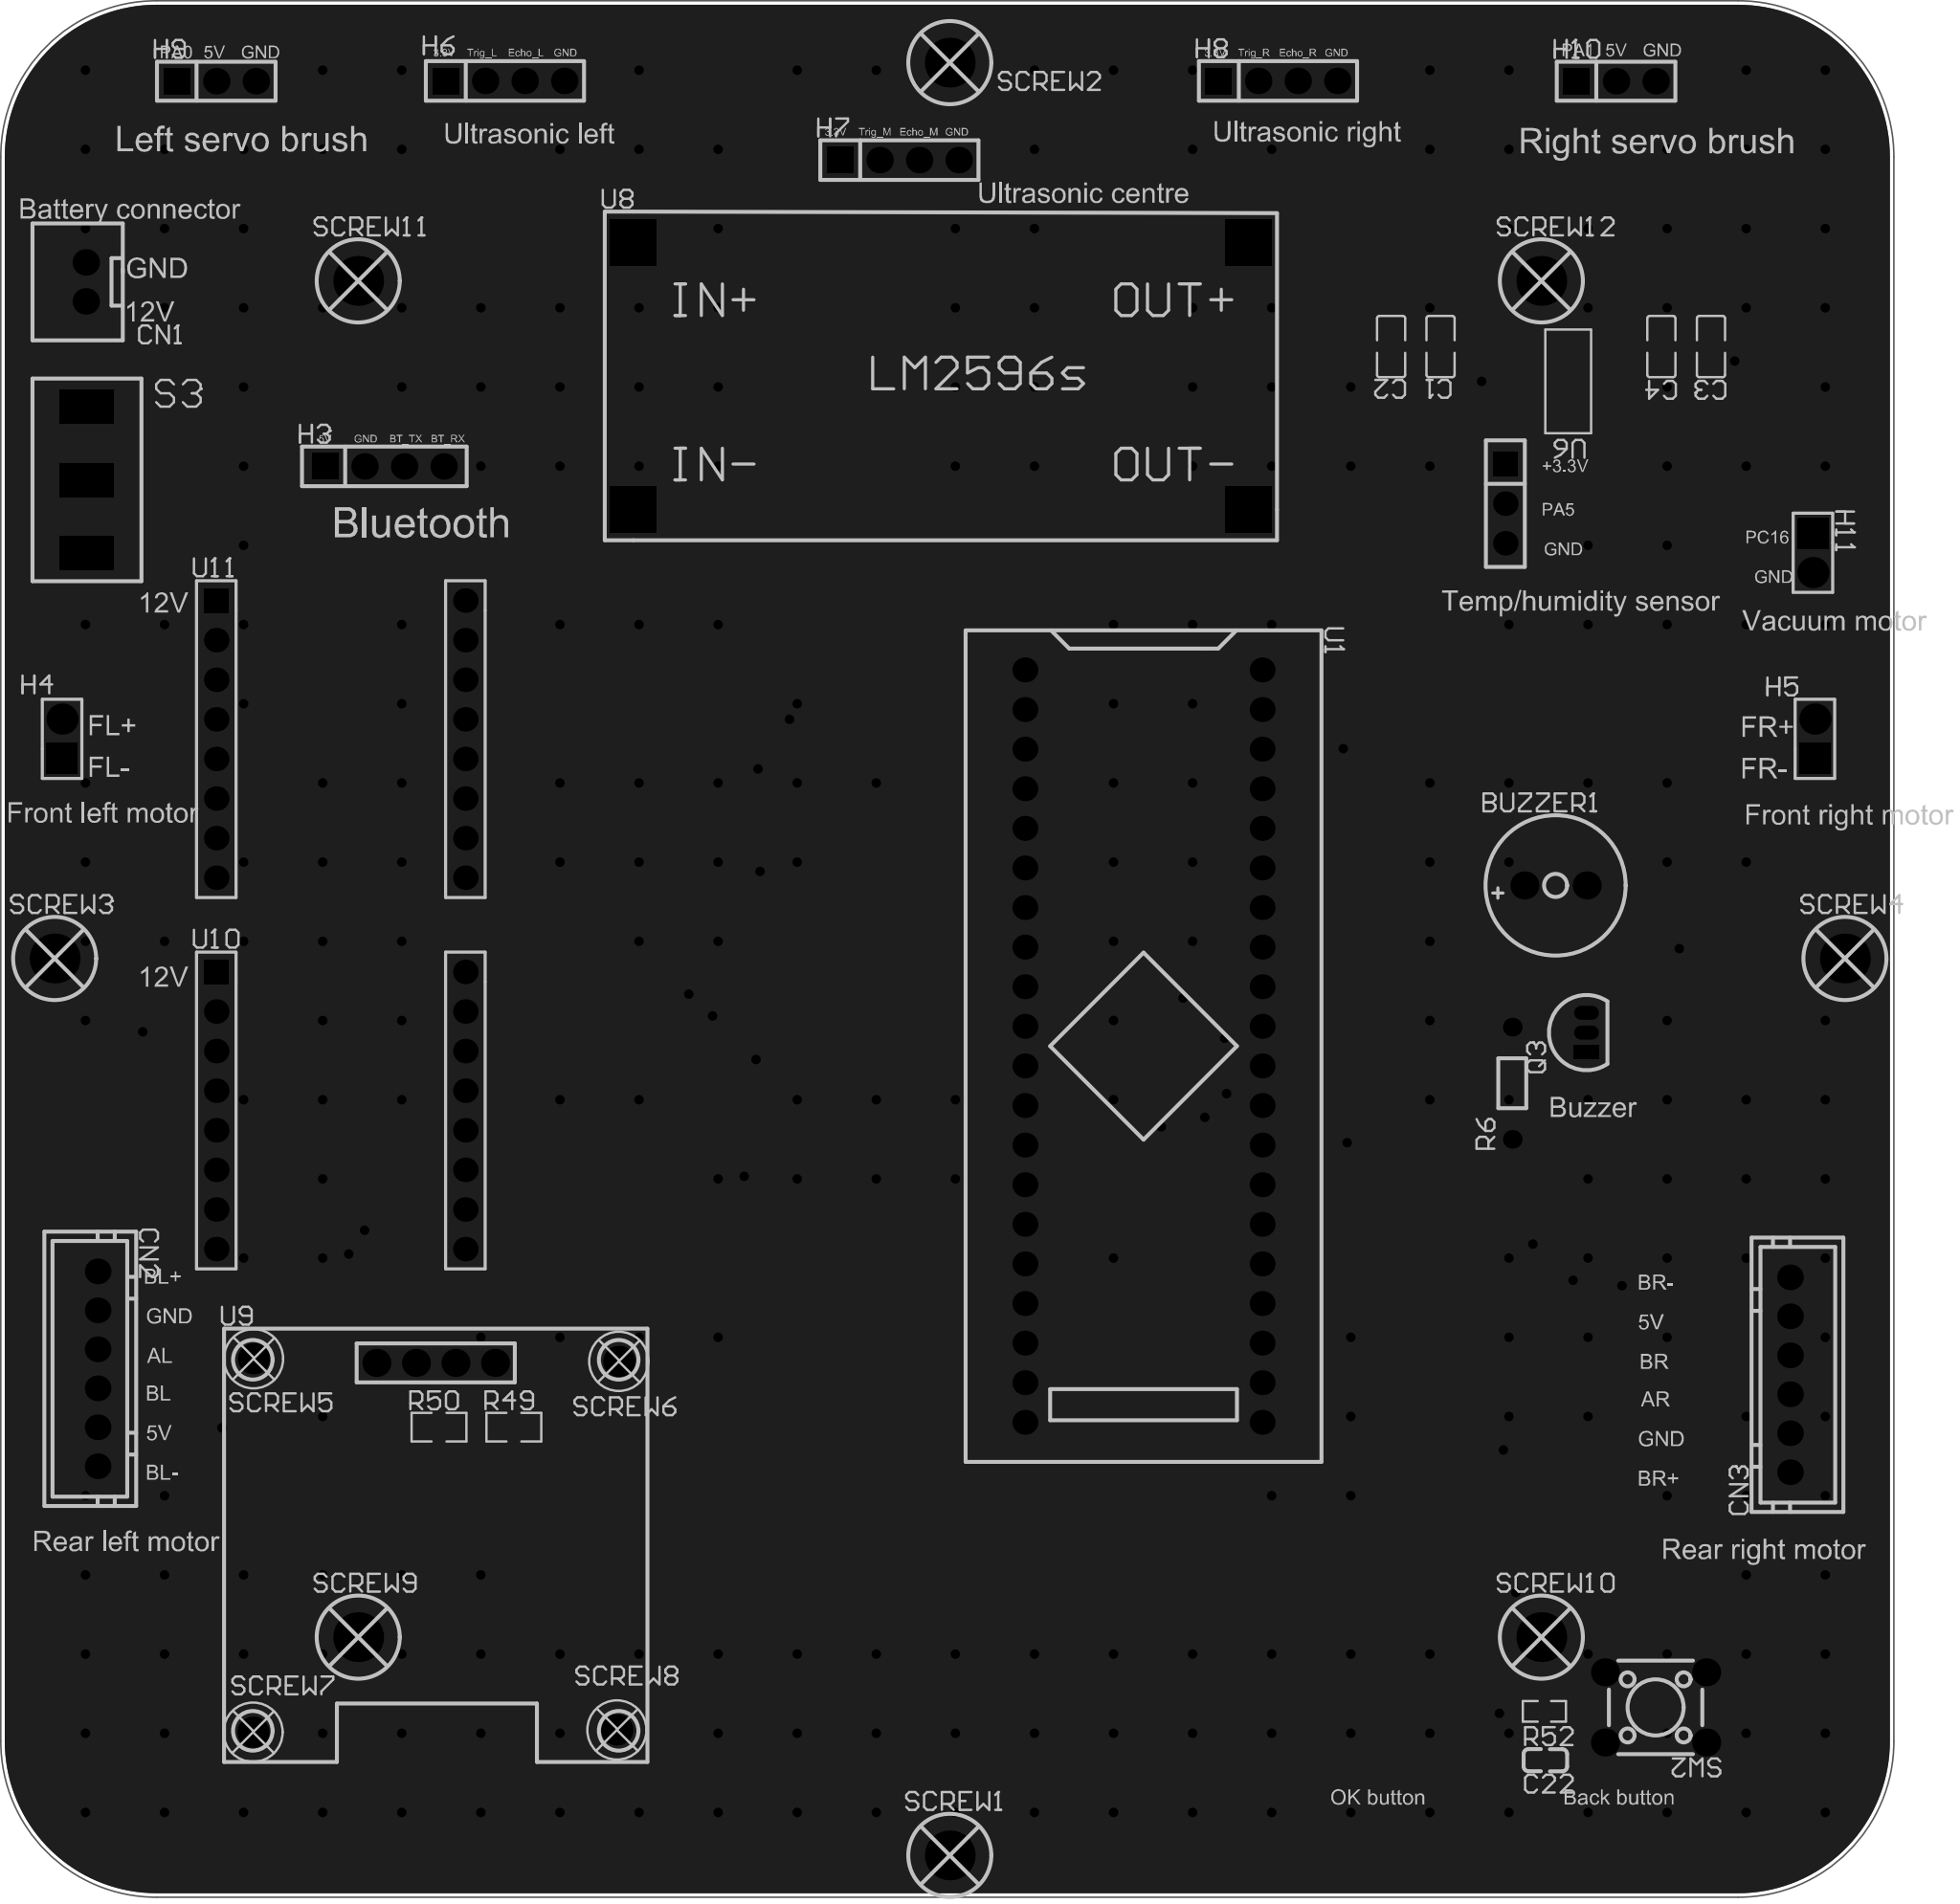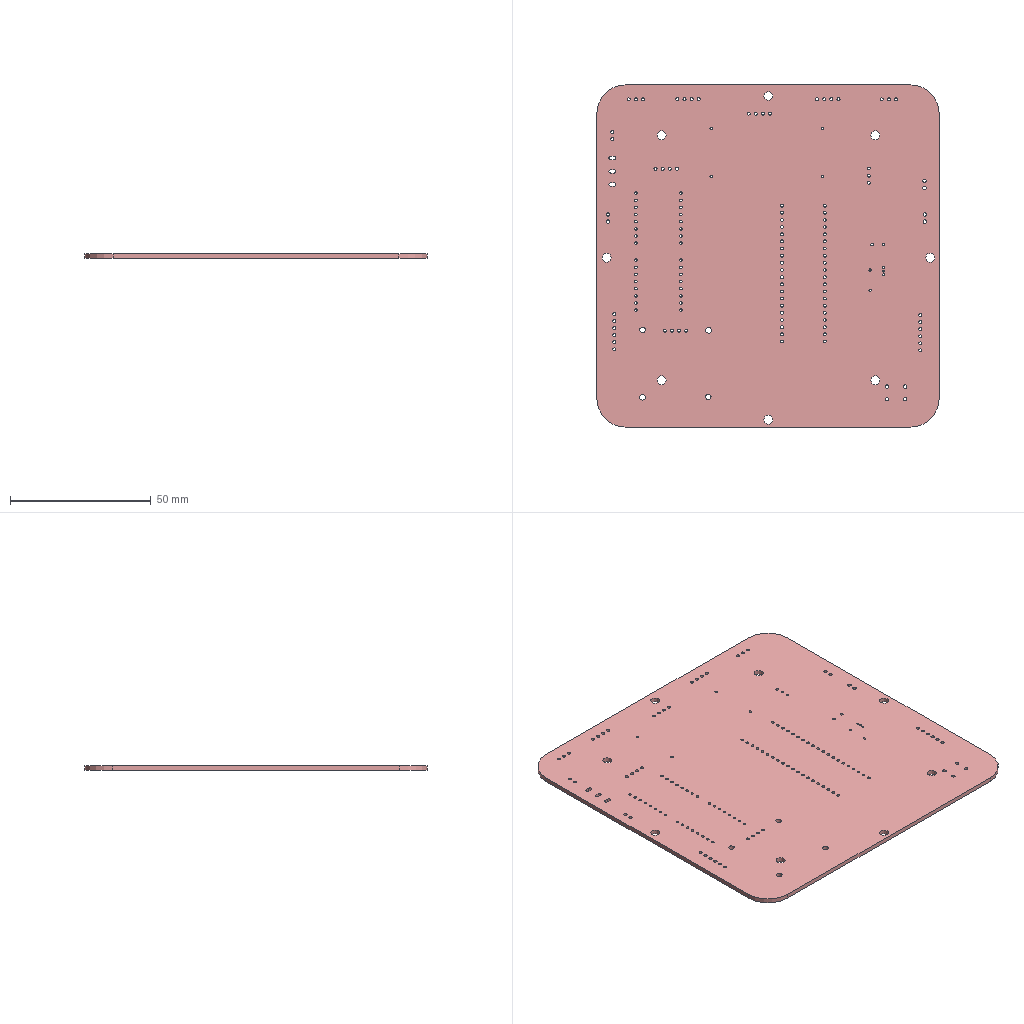Circuit board layout | Altium Designer | box 121.6 x 121.7 x 1.6 mm
Layer stack:
# Altium Designer layer stack of  (unit mm; dielectric type: 0 none, 1 core, 2 prepreg, 3 surface material)
index,name,kind,layer,copper_thickness_mm,dielectric_type,dielectric_thickness_mm,dielectric_material,dielectric_constant
0,Top Paste Mask Layer,other,,,,,,
1,Top Silkscreen Layer,other,,,,,,
2,Top Solder Mask Layer,dielectric,,,3,0.01,,3.3
3,Top Layer,copper,Top Layer,0.035,,,,
4,Dielectric1,dielectric,,,3,1.51,FR4,4.5
5,Bottom Layer,copper,Bottom Layer,0.035,,,,
6,Bottom Solder Mask Layer,dielectric,,,3,0.01,,3.3
7,Bottom Silkscreen Layer,other,,,,,,
8,Bottom Paste Mask Layer,other,,,,,,
# drill layer pairs: low layer,high layer
drill_pair,Top Layer,Bottom Layer
Part placement:
Designator,Comment,Layer,Footprint,Center-X(mm),Center-Y(mm),Rotation
CN1,XH2.54*2P_THT,TopLayer,CONN-TH_2P-P2.50-XH2.54-2P,88.519,190.373,270
CN2,Rear left motor,TopLayer,CONN-TH_XH2.54-6P,89.281,120.651,270
CN3,Rear right motor,TopLayer,CONN-TH_XH2.54-6P,197.993,120.269,90
H3,2.54-1*4P female,TopLayer,HDR-TH_4P-P2.54-V-F,107.696,178.539,0
H4,Front left motor,TopLayer,HDR-TH_2P-P2.54-V-M,86.995,161.061,90
H5,Front right motor,TopLayer,HDR-TH_2P-P2.54-V-M,199.589,161.061,90
H6,Ultrasonic left,TopLayer,HDR-TH_4P-P2.54-V-M,115.442,203.265,0
H7,Ultrasonic centre,TopLayer,HDR-TH_4P-P2.54-V-M,140.78,198.185,0
H8,Ultrasonic right,TopLayer,HDR-TH_4P-P2.54-V-M,165.101,203.265,0
H9,PZ254V-11-03P,TopLayer,HDR-TH_3P-P2.54-V-M,96.901,203.245,0
H10,PZ254V-11-03P,TopLayer,HDR-TH_3P-P2.54-V-M,186.817,203.245,0
H11,PZ254V-11-02P,TopLayer,HDR-TH_2P-P2.54-V-M,199.462,172.998,270
H12,PM254V-11-03-H85,TopLayer,HDR-TH_3P-P2.54-V-F,179.705,176.149,270
R49,4.7kΩ,TopLayer,R0805,116.016,116.908,180
R50,4.7kΩ,TopLayer,R0805,111.207,116.908,180
S3,SS12D10 switch,TopLayer,SS12D10,88.594,177.673,90
U6,AMS1117-3.3,TopLayer,SOT-223-3_L6.5-W3.4-P2.30-LS7.0-BR,183.642,183.992,180
U8,LM2596S buck module,TopLayer,LM2596S,143.446,184.34,0
U9,HS96L03W2C03,TopLayer,OLED-TH_L27.8-W27.2-P2.54_C9900033791,110.998,121.031,0
U10,TB6612 module,TopLayer,TB6612-2X8,104.901,137.222,0
U11,TB6612 module,TopLayer,TB6612-2X8,104.901,161.042,0
SCREW5,,TopLayer,M2螺丝,99.294,121.297,0
SCREW6,,TopLayer,M2螺丝,122.754,121.131,0
SCREW7,,TopLayer,M2螺丝,99.263,97.343,0
SCREW8,,TopLayer,M2螺丝,122.635,97.486,0
C1,10uF,TopLayer,C0805,175.541,186.226,270
C2,100nF,TopLayer,C0805,172.366,186.226,270
C3,10uF,TopLayer,C0805,192.913,186.226,270
C4,100nF,TopLayer,C0805,189.727,186.226,270
C22,1uF,TopLayer,C0603,182.283,95.543,0
R52,10kΩ,TopLayer,R0603,182.212,98.679,180
SCREW2,,TopLayer,M3螺丝,144.018,204.439,0
SCREW3,,TopLayer,M3螺丝,86.518,146.973,0
SCREW1,,TopLayer,M3螺丝,144.018,89.439,0
SCREW4,,TopLayer,M3螺丝,201.518,146.973,0
U1,STM32F103C8T6-Card,TopLayer,CONN-TH_L53.3-W22.9_STM32F103C8T6-CARD,156.464,141.351,270
SW2,,TopLayer,SW-TH_4P-L6.0-W6.0-P4.50-LS6.5,189.357,98.933,180
SCREW9,,TopLayer,M3螺丝,106.019,103.439,0
SCREW10,,TopLayer,M3螺丝,182.018,103.439,0
SCREW11,,TopLayer,M3螺丝,106.019,190.439,0
SCREW12,,TopLayer,M3螺丝,182.018,190.439,0
BUZZER1,2.7kHz,TopLayer,BUZ-TH_BD9.0-P4.00-D0.6-FD,182.932,151.66,0
Q3,,TopLayer,S8050_TO_92,184.917,142.218,90
R6,1K,TopLayer,Res_1/8W,180.15,138.969,90
Pad and via stacks:
# Altium Designer via and pad stacks of  (unit mm). Each distinct definition once, with the count of objects using it.
# via: kind,start_layer,end_layer,hole_mm,diameter_mm,mode(0 simple;1 top-mid-bottom;2 full stack),diameter_per_layer,count,example_net
# pad: kind,layer,hole_mm,hole_type(0 round;1 square;2 slot),plating,top_size,top_shape(1 round;2 rect;3 octagon;9 rounded rect),mid_size,bottom_size,mode,footprint,size_per_layer,count,example
pad,Multi-Layer,1.05,0,plated,1.7x1.7,1,1.7x1.7,1.7x1.7,0,CONN-TH_2P-P2.50-XH2.54-2P,,2,CN1.2
pad,Multi-Layer,1.1,0,plated,1.65x1.65,1,1.65x1.65,1.65x1.65,0,CONN-TH_XH2.54-6P,,12,CN2.1
pad,Multi-Layer,1.1,0,plated,1.7x1.7,2,1.7x1.7,1.7x1.7,0,HDR-TH_4P-P2.54-V-F,,1,H3.1
pad,Multi-Layer,1.1,0,plated,1.7x1.7,1,1.7x1.7,1.7x1.7,0,HDR-TH_4P-P2.54-V-F,,3,H3.2
pad,Multi-Layer,1.2,0,plated,2x2,2,2x2,2x2,0,HDR-TH_2P-P2.54-V-M,,3,H4.1
pad,Multi-Layer,1.2,0,plated,2x2,1,2x2,2x2,0,HDR-TH_2P-P2.54-V-M,,3,H4.2
pad,Multi-Layer,1.1,0,plated,1.7x1.7,2,1.7x1.7,1.7x1.7,0,HDR-TH_4P-P2.54-V-M,,3,H6.1
pad,Multi-Layer,1.1,0,plated,1.7x1.7,1,1.7x1.7,1.7x1.7,0,HDR-TH_4P-P2.54-V-M,,9,H6.2
pad,Multi-Layer,1.1,0,plated,1.7x1.7,2,1.7x1.7,1.7x1.7,0,HDR-TH_3P-P2.54-V-M,,2,H9.1
pad,Multi-Layer,1.1,0,plated,1.7x1.7,1,1.7x1.7,1.7x1.7,0,HDR-TH_3P-P2.54-V-M,,4,H9.2
pad,Multi-Layer,1.02,0,plated,1.575x1.575,1,1.575x1.575,1.575x1.575,0,HDR-TH_3P-P2.54-V-F,,2,H12.3
pad,Multi-Layer,1.02,0,plated,1.575x1.575,2,1.575x1.575,1.575x1.575,0,HDR-TH_3P-P2.54-V-F,,1,H12.1
pad,Multi-Layer,1.199,2,plated,2.2x3.5,2,2.2x3.5,2.2x3.5,0,SS12D10,,3,S3.3
pad,Multi-Layer,0.9144,0,plated,3x3,2,3x3,3x3,0,LM2596S,,4,U8.4
pad,Multi-Layer,1.05,0,plated,1.8x1.8,1,1.8x1.8,1.8x1.8,0,OLED-TH_L27.8-W27.2-P2.54_C9900033791,,4,U9.1
pad,Multi-Layer,0.889,0,plated,1.575x1.575,1,1.575x1.575,1.575x1.575,0,TB6612-2X8,,30,U10.8
pad,Multi-Layer,0.889,0,plated,1.575x1.575,2,1.575x1.575,1.575x1.575,0,TB6612-2X8,,2,U10.1
pad,Multi-Layer,2,0,plated,2x2,1,2x2,2x2,0,M2\u00C2\u00DD\u00CB\u00BF,,4,SCREW5.1
pad,Multi-Layer,3.2,0,plated,3.2x3.2,1,3.2x3.2,3.2x3.2,0,M3\u00C2\u00DD\u00CB\u00BF,,8,SCREW2.1
pad,Multi-Layer,1,0,plated,1.6x1.6,1,1.6x1.6,1.6x1.6,0,CONN-TH_L53.3-W22.9_STM32F103C8T6-CARD,,40,U1.1
pad,Multi-Layer,1.2,0,plated,1.8x1.8,1,1.8x1.8,1.8x1.8,0,SW-TH_4P-L6.0-W6.0-P4.50-LS6.5,,4,SW2.1
pad,Multi-Layer,1,0,plated,1.8x1.8,1,1.8x1.8,1.8x1.8,0,BUZ-TH_BD9.0-P4.00-D0.6-FD,,2,BUZZER1.1
pad,Multi-Layer,0.701,0,plated,0.8992x1.6,2,0.8992x1.6,0.8992x1.6,0,S8050_TO_92,,1,Q3.1
pad,Multi-Layer,0.701,0,plated,0.8992x1.6,1,0.8992x1.6,0.8992x1.6,0,S8050_TO_92,,2,Q3.2
pad,Multi-Layer,0.8001,0,plated,1.199x1.199,1,1.199x1.199,1.199x1.199,0,Res_1/8W,,2,R6.1
pad,Top Layer,0,0,plated,1.133x1.377,2,1.133x1.377,1.133x1.377,0,R0805,,4,R49.2
pad,Top Layer,0,0,plated,2.5x1.1,2,2.5x1.1,2.5x1.1,0,SOT-223-3_L6.5-W3.4-P2.30-LS7.0-BR,,3,U6.1
pad,Top Layer,0,0,plated,2.34x3.6,2,2.34x3.6,2.34x3.6,0,SOT-223-3_L6.5-W3.4-P2.30-LS7.0-BR,,1,U6.4
pad,Top Layer,0,0,plated,1.41x1.35,2,1.41x1.35,1.41x1.35,0,C0805,,8,C1.2
pad,Top Layer,0,0,plated,0.8x0.9,2,0.8x0.9,0.8x0.9,0,C0603,,2,C22.2
pad,Top Layer,0,0,plated,0.8065x0.864,2,0.8065x0.864,0.8065x0.864,0,R0603,,2,R52.2
via,Top Layer,Bottom Layer,0.3048,0.61,0,,306,BL
Copper pours:
name,layer,net,type(0 solid;1 hatched;2 none)
Top Layer-GND,Top Layer,GND,0
Bottom Layer-GND,Bottom Layer,GND,0